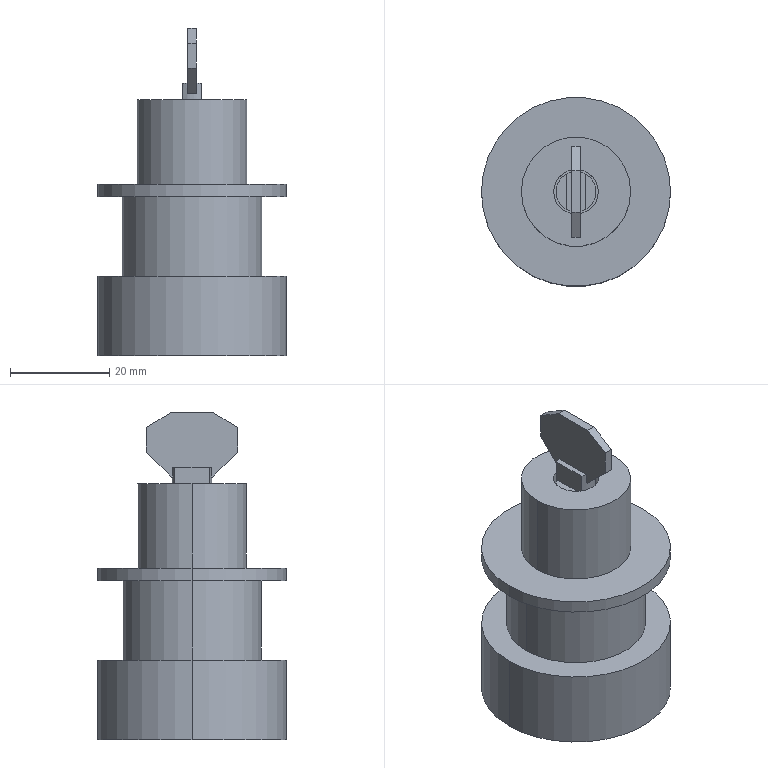Part | SolidWorks | features Boss 6, Chamfer 2, 3DProfileFeature 1, Cut 1, Extrusion 1, HoleWzd 1 | 1 solid | 35 faces | box 38 x 38 x 65.82 mm | volume 37638 mm3 | plane 23 | cylinder 12 | commonest cylinder face diameters 38 x4 8 x2 9 x2 22 x2 28 x2
STEP:
#1=CARTESIAN_POINT('',(4.,0.,50.5));
#2=VERTEX_POINT('',#1);
#3=CARTESIAN_POINT('',(2.,3.464,50.5));
#4=VERTEX_POINT('',#3);
#5=CARTESIAN_POINT('',(0.,0.,50.5));
#6=DIRECTION('',(0.,0.,1.));
#7=DIRECTION('',(1.,0.,0.));
#8=AXIS2_PLACEMENT_3D('',#5,#6,#7);
#9=CIRCLE('',#8,4.);
#10=EDGE_CURVE('',#2,#4,#9,.T.);
#11=ORIENTED_EDGE('',*,*,#10,.F.);
#12=CARTESIAN_POINT('',(4.,0.,46.5));
#13=VERTEX_POINT('',#12);
#14=CARTESIAN_POINT('',(4.,0.,50.5));
#15=DIRECTION('',(0.,0.,-1.));
#16=VECTOR('',#15,1000.);
#17=LINE('',#14,#16);
#18=EDGE_CURVE('',#2,#13,#17,.T.);
#19=ORIENTED_EDGE('',*,*,#18,.T.);
#20=CARTESIAN_POINT('',(-4.,0.,46.5));
#21=VERTEX_POINT('',#20);
#22=CARTESIAN_POINT('',(0.,0.,46.5));
#23=DIRECTION('',(0.,0.,1.));
#24=DIRECTION('',(-1.,0.,0.));
#25=AXIS2_PLACEMENT_3D('',#22,#23,#24);
#26=CIRCLE('',#25,4.);
#27=EDGE_CURVE('',#13,#21,#26,.T.);
#28=ORIENTED_EDGE('',*,*,#27,.T.);
#29=CARTESIAN_POINT('',(-4.,0.,50.5));
#30=VERTEX_POINT('',#29);
#31=CARTESIAN_POINT('',(-4.,0.,50.5));
#32=DIRECTION('',(0.,0.,-1.));
#33=VECTOR('',#32,1000.);
#34=LINE('',#31,#33);
#35=EDGE_CURVE('',#30,#21,#34,.T.);
#36=ORIENTED_EDGE('',*,*,#35,.F.);
#37=CARTESIAN_POINT('',(-2.,3.464,50.5));
#38=VERTEX_POINT('',#37);
#39=CARTESIAN_POINT('',(0.,0.,50.5));
#40=DIRECTION('',(0.,0.,1.));
#41=DIRECTION('',(1.,0.,0.));
#42=AXIS2_PLACEMENT_3D('',#39,#40,#41);
#43=CIRCLE('',#42,4.);
#44=EDGE_CURVE('',#38,#30,#43,.T.);
#45=ORIENTED_EDGE('',*,*,#44,.F.);
#46=CARTESIAN_POINT('',(-2.,3.464,54.8));
#47=VERTEX_POINT('',#46);
#48=CARTESIAN_POINT('',(-2.,3.464,54.8));
#49=DIRECTION('',(0.,0.,-1.));
#50=VECTOR('',#49,1000.);
#51=LINE('',#48,#50);
#52=EDGE_CURVE('',#47,#38,#51,.T.);
#53=ORIENTED_EDGE('',*,*,#52,.F.);
#54=CARTESIAN_POINT('',(-0.9,3.897,54.8));
#55=VERTEX_POINT('',#54);
#56=CARTESIAN_POINT('',(0.,0.,54.8));
#57=DIRECTION('',(0.,0.,1.));
#58=DIRECTION('',(1.,0.,0.));
#59=AXIS2_PLACEMENT_3D('',#56,#57,#58);
#60=CIRCLE('',#59,4.);
#61=EDGE_CURVE('',#55,#47,#60,.T.);
#62=ORIENTED_EDGE('',*,*,#61,.F.);
#63=CARTESIAN_POINT('',(-0.9,3.897,52.8));
#64=VERTEX_POINT('',#63);
#65=CARTESIAN_POINT('',(-0.9,3.897,52.8));
#66=DIRECTION('',(0.,0.,1.));
#67=VECTOR('',#66,1000.);
#68=LINE('',#65,#67);
#69=EDGE_CURVE('',#64,#55,#68,.T.);
#70=ORIENTED_EDGE('',*,*,#69,.F.);
#71=CARTESIAN_POINT('',(0.9,3.897,52.8));
#72=VERTEX_POINT('',#71);
#73=CARTESIAN_POINT('',(0.,0.,52.8));
#74=DIRECTION('',(0.,0.,1.));
#75=DIRECTION('',(1.,0.,0.));
#76=AXIS2_PLACEMENT_3D('',#73,#74,#75);
#77=CIRCLE('',#76,4.);
#78=EDGE_CURVE('',#72,#64,#77,.T.);
#79=ORIENTED_EDGE('',*,*,#78,.F.);
#80=CARTESIAN_POINT('',(0.9,3.897,54.8));
#81=VERTEX_POINT('',#80);
#82=CARTESIAN_POINT('',(0.9,3.897,52.8));
#83=DIRECTION('',(0.,0.,1.));
#84=VECTOR('',#83,1000.);
#85=LINE('',#82,#84);
#86=EDGE_CURVE('',#72,#81,#85,.T.);
#87=ORIENTED_EDGE('',*,*,#86,.T.);
#88=CARTESIAN_POINT('',(2.,3.464,54.8));
#89=VERTEX_POINT('',#88);
#90=CARTESIAN_POINT('',(0.,0.,54.8));
#91=DIRECTION('',(0.,0.,1.));
#92=DIRECTION('',(1.,0.,0.));
#93=AXIS2_PLACEMENT_3D('',#90,#91,#92);
#94=CIRCLE('',#93,4.);
#95=EDGE_CURVE('',#89,#81,#94,.T.);
#96=ORIENTED_EDGE('',*,*,#95,.F.);
#97=CARTESIAN_POINT('',(2.,3.464,54.8));
#98=DIRECTION('',(0.,0.,-1.));
#99=VECTOR('',#98,1000.);
#100=LINE('',#97,#99);
#101=EDGE_CURVE('',#89,#4,#100,.T.);
#102=ORIENTED_EDGE('',*,*,#101,.T.);
#103=EDGE_LOOP('',(#11,#19,#28,#36,#45,#53,#62,#70,#79,#87,#96,#102));
#104=FACE_OUTER_BOUND('',#103,.T.);
#105=CARTESIAN_POINT('',(0.,0.,50.5));
#106=DIRECTION('',(0.,0.,-1.));
#107=DIRECTION('',(-1.,0.,0.));
#108=AXIS2_PLACEMENT_3D('',#105,#106,#107);
#109=CYLINDRICAL_SURFACE('',#108,4.);
#110=ADVANCED_FACE('',(#104),#109,.T.);
#111=CARTESIAN_POINT('',(-4.5,0.,46.5));
#112=VERTEX_POINT('',#111);
#113=CARTESIAN_POINT('',(4.5,0.,46.5));
#114=VERTEX_POINT('',#113);
#115=CARTESIAN_POINT('',(0.,0.,46.5));
#116=DIRECTION('',(0.,0.,1.));
#117=DIRECTION('',(1.,0.,0.));
#118=AXIS2_PLACEMENT_3D('',#115,#116,#117);
#119=CIRCLE('',#118,4.5);
#120=EDGE_CURVE('',#112,#114,#119,.T.);
#121=ORIENTED_EDGE('',*,*,#120,.F.);
#122=CARTESIAN_POINT('',(-4.5,0.,51.5));
#123=VERTEX_POINT('',#122);
#124=CARTESIAN_POINT('',(-4.5,0.,51.5));
#125=DIRECTION('',(0.,0.,1.));
#126=VECTOR('',#125,1000.);
#127=LINE('',#124,#126);
#128=EDGE_CURVE('',#112,#123,#127,.T.);
#129=ORIENTED_EDGE('',*,*,#128,.T.);
#130=CARTESIAN_POINT('',(4.5,0.,51.5));
#131=VERTEX_POINT('',#130);
#132=CARTESIAN_POINT('',(0.,0.,51.5));
#133=DIRECTION('',(0.,0.,1.));
#134=DIRECTION('',(1.,0.,0.));
#135=AXIS2_PLACEMENT_3D('',#132,#133,#134);
#136=CIRCLE('',#135,4.5);
#137=EDGE_CURVE('',#123,#131,#136,.T.);
#138=ORIENTED_EDGE('',*,*,#137,.T.);
#139=CARTESIAN_POINT('',(4.5,0.,51.5));
#140=DIRECTION('',(0.,0.,1.));
#141=VECTOR('',#140,1000.);
#142=LINE('',#139,#141);
#143=EDGE_CURVE('',#114,#131,#142,.T.);
#144=ORIENTED_EDGE('',*,*,#143,.F.);
#145=EDGE_LOOP('',(#121,#129,#138,#144));
#146=FACE_OUTER_BOUND('',#145,.T.);
#147=CARTESIAN_POINT('',(0.,0.,51.5));
#148=DIRECTION('',(0.,0.,1.));
#149=DIRECTION('',(1.,0.,0.));
#150=AXIS2_PLACEMENT_3D('',#147,#148,#149);
#151=CYLINDRICAL_SURFACE('',#150,4.5);
#152=ADVANCED_FACE('',(#146),#151,.F.);
#153=CARTESIAN_POINT('',(11.,0.,51.5));
#154=VERTEX_POINT('',#153);
#155=CARTESIAN_POINT('',(-11.,0.,51.5));
#156=VERTEX_POINT('',#155);
#157=CARTESIAN_POINT('',(0.,0.,51.5));
#158=DIRECTION('',(0.,0.,1.));
#159=DIRECTION('',(1.,0.,0.));
#160=AXIS2_PLACEMENT_3D('',#157,#158,#159);
#161=CIRCLE('',#160,11.);
#162=EDGE_CURVE('',#154,#156,#161,.T.);
#163=ORIENTED_EDGE('',*,*,#162,.F.);
#164=CARTESIAN_POINT('',(11.,0.,34.5));
#165=VERTEX_POINT('',#164);
#166=CARTESIAN_POINT('',(11.,0.,51.5));
#167=DIRECTION('',(0.,0.,-1.));
#168=VECTOR('',#167,1000.);
#169=LINE('',#166,#168);
#170=EDGE_CURVE('',#154,#165,#169,.T.);
#171=ORIENTED_EDGE('',*,*,#170,.T.);
#172=CARTESIAN_POINT('',(-11.,0.,34.5));
#173=VERTEX_POINT('',#172);
#174=CARTESIAN_POINT('',(0.,0.,34.5));
#175=DIRECTION('',(0.,0.,1.));
#176=DIRECTION('',(1.,0.,0.));
#177=AXIS2_PLACEMENT_3D('',#174,#175,#176);
#178=CIRCLE('',#177,11.);
#179=EDGE_CURVE('',#165,#173,#178,.T.);
#180=ORIENTED_EDGE('',*,*,#179,.T.);
#181=CARTESIAN_POINT('',(-11.,0.,51.5));
#182=DIRECTION('',(0.,0.,-1.));
#183=VECTOR('',#182,1000.);
#184=LINE('',#181,#183);
#185=EDGE_CURVE('',#156,#173,#184,.T.);
#186=ORIENTED_EDGE('',*,*,#185,.F.);
#187=EDGE_LOOP('',(#163,#171,#180,#186));
#188=FACE_OUTER_BOUND('',#187,.T.);
#189=CARTESIAN_POINT('',(0.,0.,51.5));
#190=DIRECTION('',(0.,0.,-1.));
#191=DIRECTION('',(-1.,0.,0.));
#192=AXIS2_PLACEMENT_3D('',#189,#190,#191);
#193=CYLINDRICAL_SURFACE('',#192,11.);
#194=ADVANCED_FACE('',(#188),#193,.T.);
#195=CARTESIAN_POINT('',(19.,0.,34.5));
#196=VERTEX_POINT('',#195);
#197=CARTESIAN_POINT('',(-19.,0.,34.5));
#198=VERTEX_POINT('',#197);
#199=CARTESIAN_POINT('',(0.,0.,34.5));
#200=DIRECTION('',(0.,0.,1.));
#201=DIRECTION('',(1.,0.,0.));
#202=AXIS2_PLACEMENT_3D('',#199,#200,#201);
#203=CIRCLE('',#202,19.);
#204=EDGE_CURVE('',#196,#198,#203,.T.);
#205=ORIENTED_EDGE('',*,*,#204,.F.);
#206=CARTESIAN_POINT('',(19.,0.,32.));
#207=VERTEX_POINT('',#206);
#208=CARTESIAN_POINT('',(19.,0.,34.5));
#209=DIRECTION('',(0.,0.,-1.));
#210=VECTOR('',#209,1000.);
#211=LINE('',#208,#210);
#212=EDGE_CURVE('',#196,#207,#211,.T.);
#213=ORIENTED_EDGE('',*,*,#212,.T.);
#214=CARTESIAN_POINT('',(-19.,0.,32.));
#215=VERTEX_POINT('',#214);
#216=CARTESIAN_POINT('',(0.,0.,32.));
#217=DIRECTION('',(0.,0.,1.));
#218=DIRECTION('',(1.,0.,0.));
#219=AXIS2_PLACEMENT_3D('',#216,#217,#218);
#220=CIRCLE('',#219,19.);
#221=EDGE_CURVE('',#207,#215,#220,.T.);
#222=ORIENTED_EDGE('',*,*,#221,.T.);
#223=CARTESIAN_POINT('',(-19.,0.,34.5));
#224=DIRECTION('',(0.,0.,-1.));
#225=VECTOR('',#224,1000.);
#226=LINE('',#223,#225);
#227=EDGE_CURVE('',#198,#215,#226,.T.);
#228=ORIENTED_EDGE('',*,*,#227,.F.);
#229=EDGE_LOOP('',(#205,#213,#222,#228));
#230=FACE_OUTER_BOUND('',#229,.T.);
#231=CARTESIAN_POINT('',(0.,0.,34.5));
#232=DIRECTION('',(0.,0.,-1.));
#233=DIRECTION('',(-1.,0.,0.));
#234=AXIS2_PLACEMENT_3D('',#231,#232,#233);
#235=CYLINDRICAL_SURFACE('',#234,19.);
#236=ADVANCED_FACE('',(#230),#235,.T.);
#237=CARTESIAN_POINT('',(14.,0.,32.));
#238=VERTEX_POINT('',#237);
#239=CARTESIAN_POINT('',(-14.,0.,32.));
#240=VERTEX_POINT('',#239);
#241=CARTESIAN_POINT('',(0.,0.,32.));
#242=DIRECTION('',(0.,0.,1.));
#243=DIRECTION('',(1.,0.,0.));
#244=AXIS2_PLACEMENT_3D('',#241,#242,#243);
#245=CIRCLE('',#244,14.);
#246=EDGE_CURVE('',#238,#240,#245,.T.);
#247=ORIENTED_EDGE('',*,*,#246,.F.);
#248=CARTESIAN_POINT('',(14.,0.,16.));
#249=VERTEX_POINT('',#248);
#250=CARTESIAN_POINT('',(14.,0.,32.));
#251=DIRECTION('',(0.,0.,-1.));
#252=VECTOR('',#251,1000.);
#253=LINE('',#250,#252);
#254=EDGE_CURVE('',#238,#249,#253,.T.);
#255=ORIENTED_EDGE('',*,*,#254,.T.);
#256=CARTESIAN_POINT('',(-14.,0.,16.));
#257=VERTEX_POINT('',#256);
#258=CARTESIAN_POINT('',(0.,0.,16.));
#259=DIRECTION('',(0.,0.,1.));
#260=DIRECTION('',(1.,0.,0.));
#261=AXIS2_PLACEMENT_3D('',#258,#259,#260);
#262=CIRCLE('',#261,14.);
#263=EDGE_CURVE('',#249,#257,#262,.T.);
#264=ORIENTED_EDGE('',*,*,#263,.T.);
#265=CARTESIAN_POINT('',(-14.,0.,32.));
#266=DIRECTION('',(0.,0.,-1.));
#267=VECTOR('',#266,1000.);
#268=LINE('',#265,#267);
#269=EDGE_CURVE('',#240,#257,#268,.T.);
#270=ORIENTED_EDGE('',*,*,#269,.F.);
#271=EDGE_LOOP('',(#247,#255,#264,#270));
#272=FACE_OUTER_BOUND('',#271,.T.);
#273=CARTESIAN_POINT('',(0.,0.,32.));
#274=DIRECTION('',(0.,0.,-1.));
#275=DIRECTION('',(-1.,0.,0.));
#276=AXIS2_PLACEMENT_3D('',#273,#274,#275);
#277=CYLINDRICAL_SURFACE('',#276,14.);
#278=ADVANCED_FACE('',(#272),#277,.T.);
#279=CARTESIAN_POINT('',(19.,0.,16.));
#280=VERTEX_POINT('',#279);
#281=CARTESIAN_POINT('',(-19.,0.,16.));
#282=VERTEX_POINT('',#281);
#283=CARTESIAN_POINT('',(0.,0.,16.));
#284=DIRECTION('',(0.,0.,1.));
#285=DIRECTION('',(1.,0.,0.));
#286=AXIS2_PLACEMENT_3D('',#283,#284,#285);
#287=CIRCLE('',#286,19.);
#288=EDGE_CURVE('',#280,#282,#287,.T.);
#289=ORIENTED_EDGE('',*,*,#288,.F.);
#290=CARTESIAN_POINT('',(19.,0.,0.));
#291=VERTEX_POINT('',#290);
#292=CARTESIAN_POINT('',(19.,0.,16.));
#293=DIRECTION('',(0.,0.,-1.));
#294=VECTOR('',#293,1000.);
#295=LINE('',#292,#294);
#296=EDGE_CURVE('',#280,#291,#295,.T.);
#297=ORIENTED_EDGE('',*,*,#296,.T.);
#298=CARTESIAN_POINT('',(-19.,0.,0.));
#299=VERTEX_POINT('',#298);
#300=CARTESIAN_POINT('',(0.,0.,0.));
#301=DIRECTION('',(0.,0.,1.));
#302=DIRECTION('',(1.,0.,0.));
#303=AXIS2_PLACEMENT_3D('',#300,#301,#302);
#304=CIRCLE('',#303,19.);
#305=EDGE_CURVE('',#291,#299,#304,.T.);
#306=ORIENTED_EDGE('',*,*,#305,.T.);
#307=CARTESIAN_POINT('',(-19.,0.,16.));
#308=DIRECTION('',(0.,0.,-1.));
#309=VECTOR('',#308,1000.);
#310=LINE('',#307,#309);
#311=EDGE_CURVE('',#282,#299,#310,.T.);
#312=ORIENTED_EDGE('',*,*,#311,.F.);
#313=EDGE_LOOP('',(#289,#297,#306,#312));
#314=FACE_OUTER_BOUND('',#313,.T.);
#315=CARTESIAN_POINT('',(0.,0.,16.));
#316=DIRECTION('',(0.,0.,-1.));
#317=DIRECTION('',(-1.,0.,0.));
#318=AXIS2_PLACEMENT_3D('',#315,#316,#317);
#319=CYLINDRICAL_SURFACE('',#318,19.);
#320=ADVANCED_FACE('',(#314),#319,.T.);
#321=CARTESIAN_POINT('',(0.9,-3.897,54.8));
#322=VERTEX_POINT('',#321);
#323=CARTESIAN_POINT('',(0.9,3.897,54.8));
#324=DIRECTION('',(0.,1.,0.));
#325=VECTOR('',#324,1000.);
#326=LINE('',#323,#325);
#327=EDGE_CURVE('',#322,#81,#326,.T.);
#328=ORIENTED_EDGE('',*,*,#327,.F.);
#329=CARTESIAN_POINT('',(2.,-3.464,54.8));
#330=VERTEX_POINT('',#329);
#331=CARTESIAN_POINT('',(0.,0.,54.8));
#332=DIRECTION('',(0.,0.,1.));
#333=DIRECTION('',(1.,0.,0.));
#334=AXIS2_PLACEMENT_3D('',#331,#332,#333);
#335=CIRCLE('',#334,4.);
#336=EDGE_CURVE('',#322,#330,#335,.T.);
#337=ORIENTED_EDGE('',*,*,#336,.T.);
#338=CARTESIAN_POINT('',(2.,3.464,54.8));
#339=DIRECTION('',(0.,1.,0.));
#340=VECTOR('',#339,1000.);
#341=LINE('',#338,#340);
#342=EDGE_CURVE('',#330,#89,#341,.T.);
#343=ORIENTED_EDGE('',*,*,#342,.T.);
#344=ORIENTED_EDGE('',*,*,#95,.T.);
#345=EDGE_LOOP('',(#328,#337,#343,#344));
#346=FACE_OUTER_BOUND('',#345,.T.);
#347=CARTESIAN_POINT('',(0.,0.,54.8));
#348=DIRECTION('',(0.,0.,1.));
#349=DIRECTION('',(1.,0.,0.));
#350=AXIS2_PLACEMENT_3D('',#347,#348,#349);
#351=PLANE('',#350);
#352=ADVANCED_FACE('',(#346),#351,.T.);
#353=CARTESIAN_POINT('',(2.,-3.464,50.5));
#354=VERTEX_POINT('',#353);
#355=CARTESIAN_POINT('',(2.,3.464,50.5));
#356=DIRECTION('',(0.,1.,0.));
#357=VECTOR('',#356,1000.);
#358=LINE('',#355,#357);
#359=EDGE_CURVE('',#354,#4,#358,.T.);
#360=ORIENTED_EDGE('',*,*,#359,.F.);
#361=CARTESIAN_POINT('',(0.,0.,50.5));
#362=DIRECTION('',(0.,0.,1.));
#363=DIRECTION('',(1.,0.,0.));
#364=AXIS2_PLACEMENT_3D('',#361,#362,#363);
#365=CIRCLE('',#364,4.);
#366=EDGE_CURVE('',#354,#2,#365,.T.);
#367=ORIENTED_EDGE('',*,*,#366,.T.);
#368=ORIENTED_EDGE('',*,*,#10,.T.);
#369=EDGE_LOOP('',(#360,#367,#368));
#370=FACE_OUTER_BOUND('',#369,.T.);
#371=CARTESIAN_POINT('',(0.,0.,50.5));
#372=DIRECTION('',(0.,0.,1.));
#373=DIRECTION('',(1.,0.,0.));
#374=AXIS2_PLACEMENT_3D('',#371,#372,#373);
#375=PLANE('',#374);
#376=ADVANCED_FACE('',(#370),#375,.T.);
#377=CARTESIAN_POINT('',(0.,0.,46.5));
#378=DIRECTION('',(0.,0.,1.));
#379=DIRECTION('',(1.,0.,0.));
#380=AXIS2_PLACEMENT_3D('',#377,#378,#379);
#381=CIRCLE('',#380,4.5);
#382=EDGE_CURVE('',#114,#112,#381,.T.);
#383=ORIENTED_EDGE('',*,*,#382,.T.);
#384=ORIENTED_EDGE('',*,*,#120,.T.);
#385=EDGE_LOOP('',(#383,#384));
#386=FACE_OUTER_BOUND('',#385,.T.);
#387=CARTESIAN_POINT('',(0.,0.,46.5));
#388=DIRECTION('',(0.,0.,1.));
#389=DIRECTION('',(-1.,0.,0.));
#390=AXIS2_PLACEMENT_3D('',#387,#388,#389);
#391=CIRCLE('',#390,4.);
#392=EDGE_CURVE('',#21,#13,#391,.T.);
#393=ORIENTED_EDGE('',*,*,#392,.F.);
#394=ORIENTED_EDGE('',*,*,#27,.F.);
#395=EDGE_LOOP('',(#393,#394));
#396=FACE_BOUND('',#395,.T.);
#397=CARTESIAN_POINT('',(0.,0.,46.5));
#398=DIRECTION('',(0.,0.,-1.));
#399=DIRECTION('',(-1.,0.,0.));
#400=AXIS2_PLACEMENT_3D('',#397,#398,#399);
#401=PLANE('',#400);
#402=ADVANCED_FACE('',(#386,#396),#401,.F.);
#403=CARTESIAN_POINT('',(0.,0.,34.5));
#404=DIRECTION('',(0.,0.,1.));
#405=DIRECTION('',(1.,0.,0.));
#406=AXIS2_PLACEMENT_3D('',#403,#404,#405);
#407=CIRCLE('',#406,19.);
#408=EDGE_CURVE('',#198,#196,#407,.T.);
#409=ORIENTED_EDGE('',*,*,#408,.T.);
#410=ORIENTED_EDGE('',*,*,#204,.T.);
#411=EDGE_LOOP('',(#409,#410));
#412=FACE_OUTER_BOUND('',#411,.T.);
#413=CARTESIAN_POINT('',(0.,0.,34.5));
#414=DIRECTION('',(0.,0.,1.));
#415=DIRECTION('',(1.,0.,0.));
#416=AXIS2_PLACEMENT_3D('',#413,#414,#415);
#417=CIRCLE('',#416,11.);
#418=EDGE_CURVE('',#173,#165,#417,.T.);
#419=ORIENTED_EDGE('',*,*,#418,.F.);
#420=ORIENTED_EDGE('',*,*,#179,.F.);
#421=EDGE_LOOP('',(#419,#420));
#422=FACE_BOUND('',#421,.T.);
#423=CARTESIAN_POINT('',(0.,0.,34.5));
#424=DIRECTION('',(0.,0.,1.));
#425=DIRECTION('',(1.,0.,0.));
#426=AXIS2_PLACEMENT_3D('',#423,#424,#425);
#427=PLANE('',#426);
#428=ADVANCED_FACE('',(#412,#422),#427,.T.);
#429=CARTESIAN_POINT('',(0.,0.,16.));
#430=DIRECTION('',(0.,0.,1.));
#431=DIRECTION('',(1.,0.,0.));
#432=AXIS2_PLACEMENT_3D('',#429,#430,#431);
#433=CIRCLE('',#432,19.);
#434=EDGE_CURVE('',#282,#280,#433,.T.);
#435=ORIENTED_EDGE('',*,*,#434,.T.);
#436=ORIENTED_EDGE('',*,*,#288,.T.);
#437=EDGE_LOOP('',(#435,#436));
#438=FACE_OUTER_BOUND('',#437,.T.);
#439=CARTESIAN_POINT('',(0.,0.,16.));
#440=DIRECTION('',(0.,0.,1.));
#441=DIRECTION('',(1.,0.,0.));
#442=AXIS2_PLACEMENT_3D('',#439,#440,#441);
#443=CIRCLE('',#442,14.);
#444=EDGE_CURVE('',#257,#249,#443,.T.);
#445=ORIENTED_EDGE('',*,*,#444,.F.);
#446=ORIENTED_EDGE('',*,*,#263,.F.);
#447=EDGE_LOOP('',(#445,#446));
#448=FACE_BOUND('',#447,.T.);
#449=CARTESIAN_POINT('',(0.,0.,16.));
#450=DIRECTION('',(0.,0.,1.));
#451=DIRECTION('',(1.,0.,0.));
#452=AXIS2_PLACEMENT_3D('',#449,#450,#451);
#453=PLANE('',#452);
#454=ADVANCED_FACE('',(#438,#448),#453,.T.);
#455=ORIENTED_EDGE('',*,*,#296,.F.);
#456=ORIENTED_EDGE('',*,*,#434,.F.);
#457=ORIENTED_EDGE('',*,*,#311,.T.);
#458=CARTESIAN_POINT('',(0.,0.,0.));
#459=DIRECTION('',(0.,0.,1.));
#460=DIRECTION('',(1.,0.,0.));
#461=AXIS2_PLACEMENT_3D('',#458,#459,#460);
#462=CIRCLE('',#461,19.);
#463=EDGE_CURVE('',#299,#291,#462,.T.);
#464=ORIENTED_EDGE('',*,*,#463,.T.);
#465=EDGE_LOOP('',(#455,#456,#457,#464));
#466=FACE_OUTER_BOUND('',#465,.T.);
#467=CARTESIAN_POINT('',(0.,0.,16.));
#468=DIRECTION('',(0.,0.,-1.));
#469=DIRECTION('',(-1.,0.,0.));
#470=AXIS2_PLACEMENT_3D('',#467,#468,#469);
#471=CYLINDRICAL_SURFACE('',#470,19.);
#472=ADVANCED_FACE('',(#466),#471,.T.);
#473=ORIENTED_EDGE('',*,*,#463,.F.);
#474=ORIENTED_EDGE('',*,*,#305,.F.);
#475=EDGE_LOOP('',(#473,#474));
#476=FACE_OUTER_BOUND('',#475,.T.);
#477=CARTESIAN_POINT('',(0.,0.,0.));
#478=DIRECTION('',(0.,0.,1.));
#479=DIRECTION('',(1.,0.,0.));
#480=AXIS2_PLACEMENT_3D('',#477,#478,#479);
#481=PLANE('',#480);
#482=ADVANCED_FACE('',(#476),#481,.F.);
#483=ORIENTED_EDGE('',*,*,#254,.F.);
#484=CARTESIAN_POINT('',(0.,0.,32.));
#485=DIRECTION('',(0.,0.,1.));
#486=DIRECTION('',(1.,0.,0.));
#487=AXIS2_PLACEMENT_3D('',#484,#485,#486);
#488=CIRCLE('',#487,14.);
#489=EDGE_CURVE('',#240,#238,#488,.T.);
#490=ORIENTED_EDGE('',*,*,#489,.F.);
#491=ORIENTED_EDGE('',*,*,#269,.T.);
#492=ORIENTED_EDGE('',*,*,#444,.T.);
#493=EDGE_LOOP('',(#483,#490,#491,#492));
#494=FACE_OUTER_BOUND('',#493,.T.);
#495=CARTESIAN_POINT('',(0.,0.,32.));
#496=DIRECTION('',(0.,0.,-1.));
#497=DIRECTION('',(-1.,0.,0.));
#498=AXIS2_PLACEMENT_3D('',#495,#496,#497);
#499=CYLINDRICAL_SURFACE('',#498,14.);
#500=ADVANCED_FACE('',(#494),#499,.T.);
#501=CARTESIAN_POINT('',(0.,0.,32.));
#502=DIRECTION('',(0.,0.,1.));
#503=DIRECTION('',(1.,0.,0.));
#504=AXIS2_PLACEMENT_3D('',#501,#502,#503);
#505=CIRCLE('',#504,19.);
#506=EDGE_CURVE('',#215,#207,#505,.T.);
#507=ORIENTED_EDGE('',*,*,#506,.F.);
#508=ORIENTED_EDGE('',*,*,#221,.F.);
#509=EDGE_LOOP('',(#507,#508));
#510=FACE_OUTER_BOUND('',#509,.T.);
#511=ORIENTED_EDGE('',*,*,#489,.T.);
#512=ORIENTED_EDGE('',*,*,#246,.T.);
#513=EDGE_LOOP('',(#511,#512));
#514=FACE_BOUND('',#513,.T.);
#515=CARTESIAN_POINT('',(0.,0.,32.));
#516=DIRECTION('',(0.,0.,1.));
#517=DIRECTION('',(1.,0.,0.));
#518=AXIS2_PLACEMENT_3D('',#515,#516,#517);
#519=PLANE('',#518);
#520=ADVANCED_FACE('',(#510,#514),#519,.F.);
#521=ORIENTED_EDGE('',*,*,#212,.F.);
#522=ORIENTED_EDGE('',*,*,#408,.F.);
#523=ORIENTED_EDGE('',*,*,#227,.T.);
#524=ORIENTED_EDGE('',*,*,#506,.T.);
#525=EDGE_LOOP('',(#521,#522,#523,#524));
#526=FACE_OUTER_BOUND('',#525,.T.);
#527=CARTESIAN_POINT('',(0.,0.,34.5));
#528=DIRECTION('',(0.,0.,-1.));
#529=DIRECTION('',(-1.,0.,0.));
#530=AXIS2_PLACEMENT_3D('',#527,#528,#529);
#531=CYLINDRICAL_SURFACE('',#530,19.);
#532=ADVANCED_FACE('',(#526),#531,.T.);
#533=ORIENTED_EDGE('',*,*,#170,.F.);
#534=CARTESIAN_POINT('',(0.,0.,51.5));
#535=DIRECTION('',(0.,0.,1.));
#536=DIRECTION('',(1.,0.,0.));
#537=AXIS2_PLACEMENT_3D('',#534,#535,#536);
#538=CIRCLE('',#537,11.);
#539=EDGE_CURVE('',#156,#154,#538,.T.);
#540=ORIENTED_EDGE('',*,*,#539,.F.);
#541=ORIENTED_EDGE('',*,*,#185,.T.);
#542=ORIENTED_EDGE('',*,*,#418,.T.);
#543=EDGE_LOOP('',(#533,#540,#541,#542));
#544=FACE_OUTER_BOUND('',#543,.T.);
#545=CARTESIAN_POINT('',(0.,0.,51.5));
#546=DIRECTION('',(0.,0.,-1.));
#547=DIRECTION('',(-1.,0.,0.));
#548=AXIS2_PLACEMENT_3D('',#545,#546,#547);
#549=CYLINDRICAL_SURFACE('',#548,11.);
#550=ADVANCED_FACE('',(#544),#549,.T.);
#551=CARTESIAN_POINT('',(0.,0.,51.5));
#552=DIRECTION('',(0.,0.,1.));
#553=DIRECTION('',(1.,0.,0.));
#554=AXIS2_PLACEMENT_3D('',#551,#552,#553);
#555=CIRCLE('',#554,4.5);
#556=EDGE_CURVE('',#131,#123,#555,.T.);
#557=ORIENTED_EDGE('',*,*,#556,.F.);
#558=ORIENTED_EDGE('',*,*,#137,.F.);
#559=EDGE_LOOP('',(#557,#558));
#560=FACE_BOUND('',#559,.T.);
#561=ORIENTED_EDGE('',*,*,#539,.T.);
#562=ORIENTED_EDGE('',*,*,#162,.T.);
#563=EDGE_LOOP('',(#561,#562));
#564=FACE_OUTER_BOUND('',#563,.T.);
#565=CARTESIAN_POINT('',(0.,0.,51.5));
#566=DIRECTION('',(0.,0.,1.));
#567=DIRECTION('',(1.,0.,0.));
#568=AXIS2_PLACEMENT_3D('',#565,#566,#567);
#569=PLANE('',#568);
#570=ADVANCED_FACE('',(#560,#564),#569,.T.);
#571=ORIENTED_EDGE('',*,*,#128,.F.);
#572=ORIENTED_EDGE('',*,*,#382,.F.);
#573=ORIENTED_EDGE('',*,*,#143,.T.);
#574=ORIENTED_EDGE('',*,*,#556,.T.);
#575=EDGE_LOOP('',(#571,#572,#573,#574));
#576=FACE_OUTER_BOUND('',#575,.T.);
#577=CARTESIAN_POINT('',(0.,0.,51.5));
#578=DIRECTION('',(0.,0.,1.));
#579=DIRECTION('',(1.,0.,0.));
#580=AXIS2_PLACEMENT_3D('',#577,#578,#579);
#581=CYLINDRICAL_SURFACE('',#580,4.5);
#582=ADVANCED_FACE('',(#576),#581,.F.);
#583=ORIENTED_EDGE('',*,*,#18,.F.);
#584=ORIENTED_EDGE('',*,*,#366,.F.);
#585=CARTESIAN_POINT('',(2.,-3.464,54.8));
#586=DIRECTION('',(0.,0.,-1.));
#587=VECTOR('',#586,1000.);
#588=LINE('',#585,#587);
#589=EDGE_CURVE('',#330,#354,#588,.T.);
#590=ORIENTED_EDGE('',*,*,#589,.F.);
#591=ORIENTED_EDGE('',*,*,#336,.F.);
#592=CARTESIAN_POINT('',(0.9,-3.897,52.8));
#593=VERTEX_POINT('',#592);
#594=CARTESIAN_POINT('',(0.9,-3.897,52.8));
#595=DIRECTION('',(0.,0.,1.));
#596=VECTOR('',#595,1000.);
#597=LINE('',#594,#596);
#598=EDGE_CURVE('',#593,#322,#597,.T.);
#599=ORIENTED_EDGE('',*,*,#598,.F.);
#600=CARTESIAN_POINT('',(-0.9,-3.897,52.8));
#601=VERTEX_POINT('',#600);
#602=CARTESIAN_POINT('',(0.,0.,52.8));
#603=DIRECTION('',(0.,0.,1.));
#604=DIRECTION('',(1.,0.,0.));
#605=AXIS2_PLACEMENT_3D('',#602,#603,#604);
#606=CIRCLE('',#605,4.);
#607=EDGE_CURVE('',#601,#593,#606,.T.);
#608=ORIENTED_EDGE('',*,*,#607,.F.);
#609=CARTESIAN_POINT('',(-0.9,-3.897,54.8));
#610=VERTEX_POINT('',#609);
#611=CARTESIAN_POINT('',(-0.9,-3.897,52.8));
#612=DIRECTION('',(0.,0.,1.));
#613=VECTOR('',#612,1000.);
#614=LINE('',#611,#613);
#615=EDGE_CURVE('',#601,#610,#614,.T.);
#616=ORIENTED_EDGE('',*,*,#615,.T.);
#617=CARTESIAN_POINT('',(-2.,-3.464,54.8));
#618=VERTEX_POINT('',#617);
#619=CARTESIAN_POINT('',(0.,0.,54.8));
#620=DIRECTION('',(0.,0.,1.));
#621=DIRECTION('',(1.,0.,0.));
#622=AXIS2_PLACEMENT_3D('',#619,#620,#621);
#623=CIRCLE('',#622,4.);
#624=EDGE_CURVE('',#618,#610,#623,.T.);
#625=ORIENTED_EDGE('',*,*,#624,.F.);
#626=CARTESIAN_POINT('',(-2.,-3.464,50.5));
#627=VERTEX_POINT('',#626);
#628=CARTESIAN_POINT('',(-2.,-3.464,54.8));
#629=DIRECTION('',(0.,0.,-1.));
#630=VECTOR('',#629,1000.);
#631=LINE('',#628,#630);
#632=EDGE_CURVE('',#618,#627,#631,.T.);
#633=ORIENTED_EDGE('',*,*,#632,.T.);
#634=CARTESIAN_POINT('',(0.,0.,50.5));
#635=DIRECTION('',(0.,0.,1.));
#636=DIRECTION('',(1.,0.,0.));
#637=AXIS2_PLACEMENT_3D('',#634,#635,#636);
#638=CIRCLE('',#637,4.);
#639=EDGE_CURVE('',#30,#627,#638,.T.);
#640=ORIENTED_EDGE('',*,*,#639,.F.);
#641=ORIENTED_EDGE('',*,*,#35,.T.);
#642=ORIENTED_EDGE('',*,*,#392,.T.);
#643=EDGE_LOOP('',(#583,#584,#590,#591,#599,#608,#616,#625,#633,#640,#641,#642));
#644=FACE_OUTER_BOUND('',#643,.T.);
#645=CARTESIAN_POINT('',(0.,0.,50.5));
#646=DIRECTION('',(0.,0.,-1.));
#647=DIRECTION('',(-1.,0.,0.));
#648=AXIS2_PLACEMENT_3D('',#645,#646,#647);
#649=CYLINDRICAL_SURFACE('',#648,4.);
#650=ADVANCED_FACE('',(#644),#649,.T.);
#651=CARTESIAN_POINT('',(-2.,3.464,50.5));
#652=DIRECTION('',(0.,-1.,0.));
#653=VECTOR('',#652,1000.);
#654=LINE('',#651,#653);
#655=EDGE_CURVE('',#38,#627,#654,.T.);
#656=ORIENTED_EDGE('',*,*,#655,.F.);
#657=ORIENTED_EDGE('',*,*,#44,.T.);
#658=ORIENTED_EDGE('',*,*,#639,.T.);
#659=EDGE_LOOP('',(#656,#657,#658));
#660=FACE_OUTER_BOUND('',#659,.T.);
#661=CARTESIAN_POINT('',(0.,0.,50.5));
#662=DIRECTION('',(0.,0.,1.));
#663=DIRECTION('',(1.,0.,0.));
#664=AXIS2_PLACEMENT_3D('',#661,#662,#663);
#665=PLANE('',#664);
#666=ADVANCED_FACE('',(#660),#665,.T.);
#667=ORIENTED_EDGE('',*,*,#655,.T.);
#668=ORIENTED_EDGE('',*,*,#632,.F.);
#669=CARTESIAN_POINT('',(-2.,3.464,54.8));
#670=DIRECTION('',(0.,-1.,0.));
#671=VECTOR('',#670,1000.);
#672=LINE('',#669,#671);
#673=EDGE_CURVE('',#47,#618,#672,.T.);
#674=ORIENTED_EDGE('',*,*,#673,.F.);
#675=ORIENTED_EDGE('',*,*,#52,.T.);
#676=EDGE_LOOP('',(#667,#668,#674,#675));
#677=FACE_OUTER_BOUND('',#676,.T.);
#678=CARTESIAN_POINT('',(-2.,3.464,54.8));
#679=DIRECTION('',(1.,0.,0.));
#680=DIRECTION('',(0.,1.,0.));
#681=AXIS2_PLACEMENT_3D('',#678,#679,#680);
#682=PLANE('',#681);
#683=ADVANCED_FACE('',(#677),#682,.F.);
#684=ORIENTED_EDGE('',*,*,#359,.T.);
#685=ORIENTED_EDGE('',*,*,#101,.F.);
#686=ORIENTED_EDGE('',*,*,#342,.F.);
#687=ORIENTED_EDGE('',*,*,#589,.T.);
#688=EDGE_LOOP('',(#684,#685,#686,#687));
#689=FACE_OUTER_BOUND('',#688,.T.);
#690=CARTESIAN_POINT('',(2.,3.464,54.8));
#691=DIRECTION('',(-1.,0.,0.));
#692=DIRECTION('',(0.,-1.,0.));
#693=AXIS2_PLACEMENT_3D('',#690,#691,#692);
#694=PLANE('',#693);
#695=ADVANCED_FACE('',(#689),#694,.F.);
#696=CARTESIAN_POINT('',(-0.9,3.897,54.8));
#697=DIRECTION('',(0.,-1.,0.));
#698=VECTOR('',#697,1000.);
#699=LINE('',#696,#698);
#700=EDGE_CURVE('',#55,#610,#699,.T.);
#701=ORIENTED_EDGE('',*,*,#700,.F.);
#702=ORIENTED_EDGE('',*,*,#61,.T.);
#703=ORIENTED_EDGE('',*,*,#673,.T.);
#704=ORIENTED_EDGE('',*,*,#624,.T.);
#705=EDGE_LOOP('',(#701,#702,#703,#704));
#706=FACE_OUTER_BOUND('',#705,.T.);
#707=CARTESIAN_POINT('',(0.,0.,54.8));
#708=DIRECTION('',(0.,0.,1.));
#709=DIRECTION('',(1.,0.,0.));
#710=AXIS2_PLACEMENT_3D('',#707,#708,#709);
#711=PLANE('',#710);
#712=ADVANCED_FACE('',(#706),#711,.T.);
#713=CARTESIAN_POINT('',(-0.9,4.15,52.8));
#714=VERTEX_POINT('',#713);
#715=CARTESIAN_POINT('',(-0.9,9.15,52.8));
#716=DIRECTION('',(0.,-1.,0.));
#717=VECTOR('',#716,1000.);
#718=LINE('',#715,#717);
#719=EDGE_CURVE('',#714,#64,#718,.T.);
#720=ORIENTED_EDGE('',*,*,#719,.F.);
#721=CARTESIAN_POINT('',(0.9,4.15,52.8));
#722=VERTEX_POINT('',#721);
#723=CARTESIAN_POINT('',(0.9,4.15,52.8));
#724=DIRECTION('',(1.,0.,0.));
#725=VECTOR('',#724,1000.);
#726=LINE('',#723,#725);
#727=EDGE_CURVE('',#714,#722,#726,.T.);
#728=ORIENTED_EDGE('',*,*,#727,.T.);
#729=CARTESIAN_POINT('',(0.9,9.15,52.8));
#730=DIRECTION('',(0.,1.,0.));
#731=VECTOR('',#730,1000.);
#732=LINE('',#729,#731);
#733=EDGE_CURVE('',#72,#722,#732,.T.);
#734=ORIENTED_EDGE('',*,*,#733,.F.);
#735=ORIENTED_EDGE('',*,*,#78,.T.);
#736=EDGE_LOOP('',(#720,#728,#734,#735));
#737=FACE_OUTER_BOUND('',#736,.T.);
#738=CARTESIAN_POINT('',(-0.9,9.15,52.8));
#739=DIRECTION('',(0.,0.,-1.));
#740=DIRECTION('',(-1.,0.,0.));
#741=AXIS2_PLACEMENT_3D('',#738,#739,#740);
#742=PLANE('',#741);
#743=ADVANCED_FACE('',(#737),#742,.T.);
#744=CARTESIAN_POINT('',(0.9,-4.15,52.8));
#745=VERTEX_POINT('',#744);
#746=CARTESIAN_POINT('',(0.9,9.15,52.8));
#747=DIRECTION('',(0.,1.,0.));
#748=VECTOR('',#747,1000.);
#749=LINE('',#746,#748);
#750=EDGE_CURVE('',#745,#593,#749,.T.);
#751=ORIENTED_EDGE('',*,*,#750,.F.);
#752=CARTESIAN_POINT('',(-0.9,-4.15,52.8));
#753=VERTEX_POINT('',#752);
#754=CARTESIAN_POINT('',(-0.9,-4.15,52.8));
#755=DIRECTION('',(-1.,0.,0.));
#756=VECTOR('',#755,1000.);
#757=LINE('',#754,#756);
#758=EDGE_CURVE('',#745,#753,#757,.T.);
#759=ORIENTED_EDGE('',*,*,#758,.T.);
#760=CARTESIAN_POINT('',(-0.9,9.15,52.8));
#761=DIRECTION('',(0.,-1.,0.));
#762=VECTOR('',#761,1000.);
#763=LINE('',#760,#762);
#764=EDGE_CURVE('',#601,#753,#763,.T.);
#765=ORIENTED_EDGE('',*,*,#764,.F.);
#766=ORIENTED_EDGE('',*,*,#607,.T.);
#767=EDGE_LOOP('',(#751,#759,#765,#766));
#768=FACE_OUTER_BOUND('',#767,.T.);
#769=CARTESIAN_POINT('',(-0.9,9.15,52.8));
#770=DIRECTION('',(0.,0.,-1.));
#771=DIRECTION('',(-1.,0.,0.));
#772=AXIS2_PLACEMENT_3D('',#769,#770,#771);
#773=PLANE('',#772);
#774=ADVANCED_FACE('',(#768),#773,.T.);
#775=ORIENTED_EDGE('',*,*,#764,.T.);
#776=CARTESIAN_POINT('',(-0.9,-9.15,57.8));
#777=VERTEX_POINT('',#776);
#778=CARTESIAN_POINT('',(-0.9,-9.15,57.8));
#779=DIRECTION('',(0.,-0.7071,0.7071));
#780=VECTOR('',#779,1000.);
#781=LINE('',#778,#780);
#782=EDGE_CURVE('',#753,#777,#781,.T.);
#783=ORIENTED_EDGE('',*,*,#782,.T.);
#784=CARTESIAN_POINT('',(-0.9,-9.15,62.82));
#785=VERTEX_POINT('',#784);
#786=CARTESIAN_POINT('',(-0.9,-9.15,65.82));
#787=DIRECTION('',(0.,0.,-1.));
#788=VECTOR('',#787,1000.);
#789=LINE('',#786,#788);
#790=EDGE_CURVE('',#785,#777,#789,.T.);
#791=ORIENTED_EDGE('',*,*,#790,.F.);
#792=CARTESIAN_POINT('',(-0.9,-4.15,65.82));
#793=VERTEX_POINT('',#792);
#794=CARTESIAN_POINT('',(-0.9,-4.15,65.82));
#795=DIRECTION('',(0.,0.8575,0.5145));
#796=VECTOR('',#795,1000.);
#797=LINE('',#794,#796);
#798=EDGE_CURVE('',#785,#793,#797,.T.);
#799=ORIENTED_EDGE('',*,*,#798,.T.);
#800=CARTESIAN_POINT('',(-0.9,4.15,65.82));
#801=VERTEX_POINT('',#800);
#802=CARTESIAN_POINT('',(-0.9,9.15,65.82));
#803=DIRECTION('',(0.,-1.,0.));
#804=VECTOR('',#803,1000.);
#805=LINE('',#802,#804);
#806=EDGE_CURVE('',#801,#793,#805,.T.);
#807=ORIENTED_EDGE('',*,*,#806,.F.);
#808=CARTESIAN_POINT('',(-0.9,9.15,62.82));
#809=VERTEX_POINT('',#808);
#810=CARTESIAN_POINT('',(-0.9,4.15,65.82));
#811=DIRECTION('',(0.,0.8575,-0.5145));
#812=VECTOR('',#811,1000.);
#813=LINE('',#810,#812);
#814=EDGE_CURVE('',#801,#809,#813,.T.);
#815=ORIENTED_EDGE('',*,*,#814,.T.);
#816=CARTESIAN_POINT('',(-0.9,9.15,57.8));
#817=VERTEX_POINT('',#816);
#818=CARTESIAN_POINT('',(-0.9,9.15,65.82));
#819=DIRECTION('',(0.,0.,-1.));
#820=VECTOR('',#819,1000.);
#821=LINE('',#818,#820);
#822=EDGE_CURVE('',#809,#817,#821,.T.);
#823=ORIENTED_EDGE('',*,*,#822,.T.);
#824=CARTESIAN_POINT('',(-0.9,9.15,57.8));
#825=DIRECTION('',(0.,-0.7071,-0.7071));
#826=VECTOR('',#825,1000.);
#827=LINE('',#824,#826);
#828=EDGE_CURVE('',#817,#714,#827,.T.);
#829=ORIENTED_EDGE('',*,*,#828,.T.);
#830=ORIENTED_EDGE('',*,*,#719,.T.);
#831=ORIENTED_EDGE('',*,*,#69,.T.);
#832=ORIENTED_EDGE('',*,*,#700,.T.);
#833=ORIENTED_EDGE('',*,*,#615,.F.);
#834=EDGE_LOOP('',(#775,#783,#791,#799,#807,#815,#823,#829,#830,#831,#832,#833));
#835=FACE_OUTER_BOUND('',#834,.T.);
#836=CARTESIAN_POINT('',(-0.9,9.15,65.82));
#837=DIRECTION('',(1.,0.,0.));
#838=DIRECTION('',(0.,1.,0.));
#839=AXIS2_PLACEMENT_3D('',#836,#837,#838);
#840=PLANE('',#839);
#841=ADVANCED_FACE('',(#835),#840,.F.);
#842=CARTESIAN_POINT('',(0.9,-9.15,62.82));
#843=VERTEX_POINT('',#842);
#844=CARTESIAN_POINT('',(0.9,-9.15,57.8));
#845=VERTEX_POINT('',#844);
#846=CARTESIAN_POINT('',(0.9,-9.15,65.82));
#847=DIRECTION('',(0.,0.,-1.));
#848=VECTOR('',#847,1000.);
#849=LINE('',#846,#848);
#850=EDGE_CURVE('',#843,#845,#849,.T.);
#851=ORIENTED_EDGE('',*,*,#850,.T.);
#852=CARTESIAN_POINT('',(0.9,-9.15,57.8));
#853=DIRECTION('',(0.,0.7071,-0.7071));
#854=VECTOR('',#853,1000.);
#855=LINE('',#852,#854);
#856=EDGE_CURVE('',#845,#745,#855,.T.);
#857=ORIENTED_EDGE('',*,*,#856,.T.);
#858=ORIENTED_EDGE('',*,*,#750,.T.);
#859=ORIENTED_EDGE('',*,*,#598,.T.);
#860=ORIENTED_EDGE('',*,*,#327,.T.);
#861=ORIENTED_EDGE('',*,*,#86,.F.);
#862=ORIENTED_EDGE('',*,*,#733,.T.);
#863=CARTESIAN_POINT('',(0.9,9.15,57.8));
#864=VERTEX_POINT('',#863);
#865=CARTESIAN_POINT('',(0.9,9.15,57.8));
#866=DIRECTION('',(0.,0.7071,0.7071));
#867=VECTOR('',#866,1000.);
#868=LINE('',#865,#867);
#869=EDGE_CURVE('',#722,#864,#868,.T.);
#870=ORIENTED_EDGE('',*,*,#869,.T.);
#871=CARTESIAN_POINT('',(0.9,9.15,62.82));
#872=VERTEX_POINT('',#871);
#873=CARTESIAN_POINT('',(0.9,9.15,65.82));
#874=DIRECTION('',(0.,0.,-1.));
#875=VECTOR('',#874,1000.);
#876=LINE('',#873,#875);
#877=EDGE_CURVE('',#872,#864,#876,.T.);
#878=ORIENTED_EDGE('',*,*,#877,.F.);
#879=CARTESIAN_POINT('',(0.9,4.15,65.82));
#880=VERTEX_POINT('',#879);
#881=CARTESIAN_POINT('',(0.9,4.15,65.82));
#882=DIRECTION('',(0.,-0.8575,0.5145));
#883=VECTOR('',#882,1000.);
#884=LINE('',#881,#883);
#885=EDGE_CURVE('',#872,#880,#884,.T.);
#886=ORIENTED_EDGE('',*,*,#885,.T.);
#887=CARTESIAN_POINT('',(0.9,-4.15,65.82));
#888=VERTEX_POINT('',#887);
#889=CARTESIAN_POINT('',(0.9,9.15,65.82));
#890=DIRECTION('',(0.,1.,0.));
#891=VECTOR('',#890,1000.);
#892=LINE('',#889,#891);
#893=EDGE_CURVE('',#888,#880,#892,.T.);
#894=ORIENTED_EDGE('',*,*,#893,.F.);
#895=CARTESIAN_POINT('',(0.9,-4.15,65.82));
#896=DIRECTION('',(0.,-0.8575,-0.5145));
#897=VECTOR('',#896,1000.);
#898=LINE('',#895,#897);
#899=EDGE_CURVE('',#888,#843,#898,.T.);
#900=ORIENTED_EDGE('',*,*,#899,.T.);
#901=EDGE_LOOP('',(#851,#857,#858,#859,#860,#861,#862,#870,#878,#886,#894,#900));
#902=FACE_OUTER_BOUND('',#901,.T.);
#903=CARTESIAN_POINT('',(0.9,9.15,65.82));
#904=DIRECTION('',(-1.,0.,0.));
#905=DIRECTION('',(0.,-1.,0.));
#906=AXIS2_PLACEMENT_3D('',#903,#904,#905);
#907=PLANE('',#906);
#908=ADVANCED_FACE('',(#902),#907,.F.);
#909=ORIENTED_EDGE('',*,*,#877,.T.);
#910=CARTESIAN_POINT('',(-0.9,9.15,57.8));
#911=DIRECTION('',(-1.,0.,0.));
#912=VECTOR('',#911,1000.);
#913=LINE('',#910,#912);
#914=EDGE_CURVE('',#864,#817,#913,.T.);
#915=ORIENTED_EDGE('',*,*,#914,.T.);
#916=ORIENTED_EDGE('',*,*,#822,.F.);
#917=CARTESIAN_POINT('',(-0.9,9.15,62.82));
#918=DIRECTION('',(1.,0.,0.));
#919=VECTOR('',#918,1000.);
#920=LINE('',#917,#919);
#921=EDGE_CURVE('',#809,#872,#920,.T.);
#922=ORIENTED_EDGE('',*,*,#921,.T.);
#923=EDGE_LOOP('',(#909,#915,#916,#922));
#924=FACE_OUTER_BOUND('',#923,.T.);
#925=CARTESIAN_POINT('',(-0.9,9.15,65.82));
#926=DIRECTION('',(0.,-1.,0.));
#927=DIRECTION('',(0.,0.,-1.));
#928=AXIS2_PLACEMENT_3D('',#925,#926,#927);
#929=PLANE('',#928);
#930=ADVANCED_FACE('',(#924),#929,.F.);
#931=ORIENTED_EDGE('',*,*,#790,.T.);
#932=CARTESIAN_POINT('',(0.9,-9.15,57.8));
#933=DIRECTION('',(1.,0.,0.));
#934=VECTOR('',#933,1000.);
#935=LINE('',#932,#934);
#936=EDGE_CURVE('',#777,#845,#935,.T.);
#937=ORIENTED_EDGE('',*,*,#936,.T.);
#938=ORIENTED_EDGE('',*,*,#850,.F.);
#939=CARTESIAN_POINT('',(0.9,-9.15,62.82));
#940=DIRECTION('',(-1.,0.,0.));
#941=VECTOR('',#940,1000.);
#942=LINE('',#939,#941);
#943=EDGE_CURVE('',#843,#785,#942,.T.);
#944=ORIENTED_EDGE('',*,*,#943,.T.);
#945=EDGE_LOOP('',(#931,#937,#938,#944));
#946=FACE_OUTER_BOUND('',#945,.T.);
#947=CARTESIAN_POINT('',(0.9,-9.15,65.82));
#948=DIRECTION('',(0.,1.,0.));
#949=DIRECTION('',(0.,0.,1.));
#950=AXIS2_PLACEMENT_3D('',#947,#948,#949);
#951=PLANE('',#950);
#952=ADVANCED_FACE('',(#946),#951,.F.);
#953=ORIENTED_EDGE('',*,*,#806,.T.);
#954=CARTESIAN_POINT('',(-0.9,-4.15,65.82));
#955=DIRECTION('',(1.,0.,0.));
#956=VECTOR('',#955,1000.);
#957=LINE('',#954,#956);
#958=EDGE_CURVE('',#793,#888,#957,.T.);
#959=ORIENTED_EDGE('',*,*,#958,.T.);
#960=ORIENTED_EDGE('',*,*,#893,.T.);
#961=CARTESIAN_POINT('',(-0.9,4.15,65.82));
#962=DIRECTION('',(-1.,0.,0.));
#963=VECTOR('',#962,1000.);
#964=LINE('',#961,#963);
#965=EDGE_CURVE('',#880,#801,#964,.T.);
#966=ORIENTED_EDGE('',*,*,#965,.T.);
#967=EDGE_LOOP('',(#953,#959,#960,#966));
#968=FACE_OUTER_BOUND('',#967,.T.);
#969=CARTESIAN_POINT('',(-0.9,9.15,65.82));
#970=DIRECTION('',(0.,0.,-1.));
#971=DIRECTION('',(-1.,0.,0.));
#972=AXIS2_PLACEMENT_3D('',#969,#970,#971);
#973=PLANE('',#972);
#974=ADVANCED_FACE('',(#968),#973,.F.);
#975=ORIENTED_EDGE('',*,*,#798,.F.);
#976=ORIENTED_EDGE('',*,*,#943,.F.);
#977=ORIENTED_EDGE('',*,*,#899,.F.);
#978=ORIENTED_EDGE('',*,*,#958,.F.);
#979=EDGE_LOOP('',(#975,#976,#977,#978));
#980=FACE_OUTER_BOUND('',#979,.T.);
#981=CARTESIAN_POINT('',(-0.9,-4.15,65.82));
#982=DIRECTION('',(0.,0.5145,-0.8575));
#983=DIRECTION('',(0.,0.8575,0.5145));
#984=AXIS2_PLACEMENT_3D('',#981,#982,#983);
#985=PLANE('',#984);
#986=ADVANCED_FACE('',(#980),#985,.F.);
#987=ORIENTED_EDGE('',*,*,#885,.F.);
#988=ORIENTED_EDGE('',*,*,#921,.F.);
#989=ORIENTED_EDGE('',*,*,#814,.F.);
#990=ORIENTED_EDGE('',*,*,#965,.F.);
#991=EDGE_LOOP('',(#987,#988,#989,#990));
#992=FACE_OUTER_BOUND('',#991,.T.);
#993=CARTESIAN_POINT('',(-0.9,4.15,65.82));
#994=DIRECTION('',(0.,-0.5145,-0.8575));
#995=DIRECTION('',(0.,0.8575,-0.5145));
#996=AXIS2_PLACEMENT_3D('',#993,#994,#995);
#997=PLANE('',#996);
#998=ADVANCED_FACE('',(#992),#997,.F.);
#999=ORIENTED_EDGE('',*,*,#782,.F.);
#1000=ORIENTED_EDGE('',*,*,#758,.F.);
#1001=ORIENTED_EDGE('',*,*,#856,.F.);
#1002=ORIENTED_EDGE('',*,*,#936,.F.);
#1003=EDGE_LOOP('',(#999,#1000,#1001,#1002));
#1004=FACE_OUTER_BOUND('',#1003,.T.);
#1005=CARTESIAN_POINT('',(0.9,-9.15,57.8));
#1006=DIRECTION('',(0.,-0.7071,-0.7071));
#1007=DIRECTION('',(0.,0.7071,-0.7071));
#1008=AXIS2_PLACEMENT_3D('',#1005,#1006,#1007);
#1009=PLANE('',#1008);
#1010=ADVANCED_FACE('',(#1004),#1009,.T.);
#1011=ORIENTED_EDGE('',*,*,#869,.F.);
#1012=ORIENTED_EDGE('',*,*,#727,.F.);
#1013=ORIENTED_EDGE('',*,*,#828,.F.);
#1014=ORIENTED_EDGE('',*,*,#914,.F.);
#1015=EDGE_LOOP('',(#1011,#1012,#1013,#1014));
#1016=FACE_OUTER_BOUND('',#1015,.T.);
#1017=CARTESIAN_POINT('',(-0.9,9.15,57.8));
#1018=DIRECTION('',(0.,0.7071,-0.7071));
#1019=DIRECTION('',(0.,0.7071,0.7071));
#1020=AXIS2_PLACEMENT_3D('',#1017,#1018,#1019);
#1021=PLANE('',#1020);
#1022=ADVANCED_FACE('',(#1016),#1021,.T.);
#1023=CLOSED_SHELL('',(#110,#152,#194,#236,#278,#320,#352,#376,#402,#428,#454,#472,#482,#500,#520,#532,#550,#570,#582,#650,#666,#683,#695,#712,#743,#774,#841,#908,#930,#952,#974,#986,#998,#1010,#1022));
#1024=MANIFOLD_SOLID_BREP('',#1023);
#1025=CARTESIAN_POINT('',(0.,0.,0.));
#1026=DIRECTION('',(0.,0.,1.));
#1027=DIRECTION('',(1.,0.,0.));
#1028=AXIS2_PLACEMENT_3D('',#1025,#1026,#1027);
#1029=(LENGTH_UNIT()NAMED_UNIT(*)SI_UNIT(.MILLI.,.METRE.));
#1030=UNCERTAINTY_MEASURE_WITH_UNIT(LENGTH_MEASURE(0.00001),#1029,'','');
#1031=(NAMED_UNIT(*)PLANE_ANGLE_UNIT()SI_UNIT($,.RADIAN.));
#1032=(NAMED_UNIT(*)SI_UNIT($,.STERADIAN.)SOLID_ANGLE_UNIT());
#1033=(GEOMETRIC_REPRESENTATION_CONTEXT(3)GLOBAL_UNCERTAINTY_ASSIGNED_CONTEXT((#1030))GLOBAL_UNIT_ASSIGNED_CONTEXT((#1029,#1031,#1032))REPRESENTATION_CONTEXT('',''));
#1034=ADVANCED_BREP_SHAPE_REPRESENTATION('',(#1024,#1028),#1033);